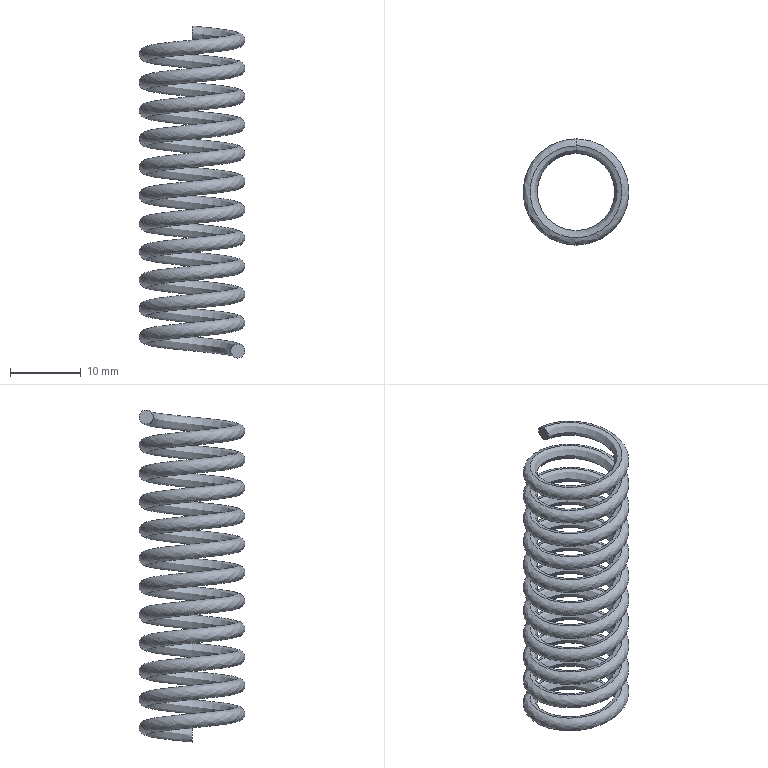Part | SolidWorks | features 3DProfileFeature 1, Helix 1, RefAxis 1, Sweep 1 | 1 solid | 4 faces | box 15 x 15 x 47 mm | volume 1444 mm3 | spline 2 | plane 2